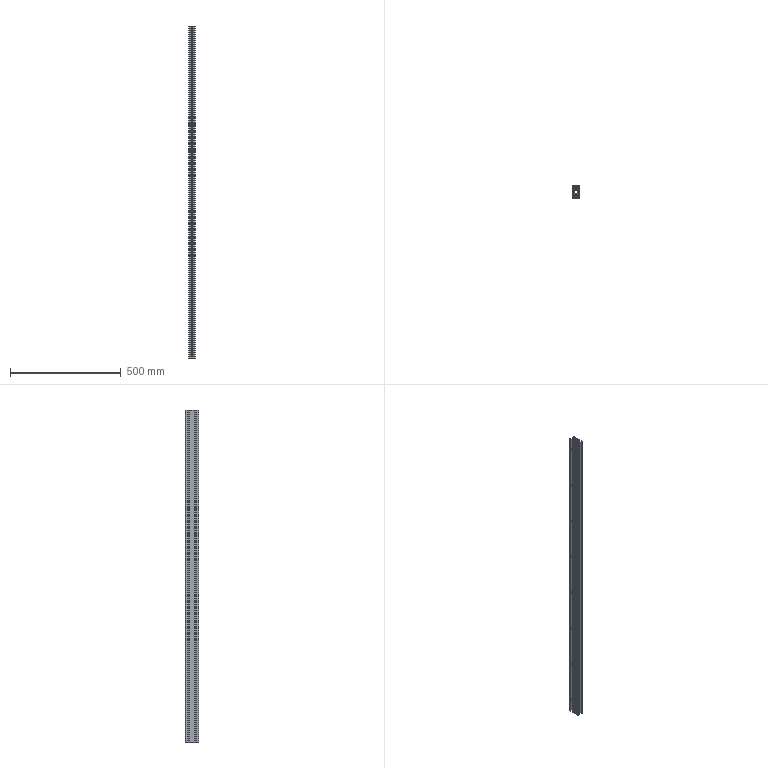Part | STEP file | Industrial aluminium profile 3060 | 1 solid | 1064 faces | box 30 x 60 x 1500 mm | volume 776079 mm3 | cylinder 650 | plane 414 | commonest cylinder face diameters 0.6 x348 1.5 x108 6.8 x90 8.4 x48 15 x32 2 x16